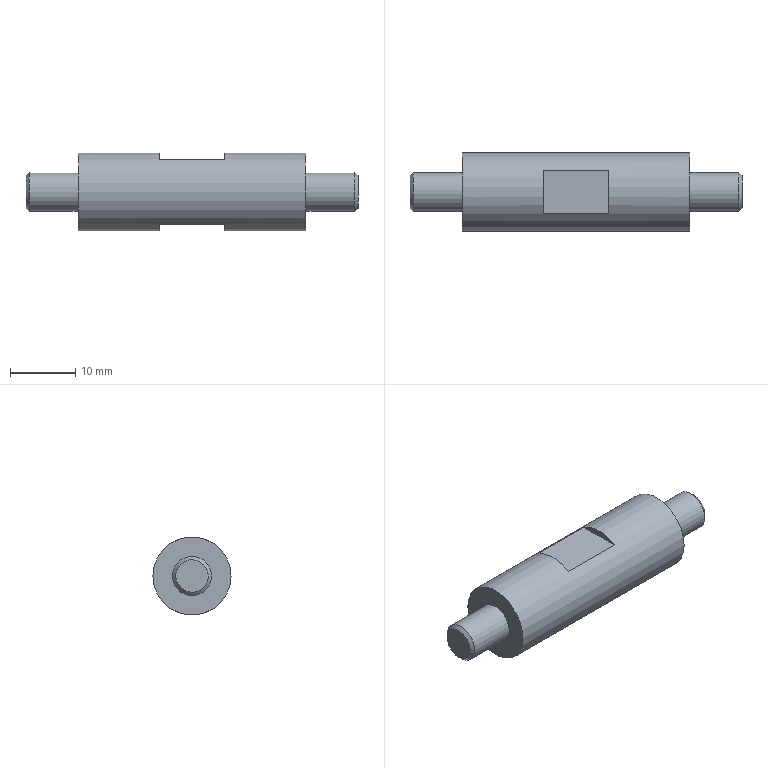Part | NX | features BREP 1 | 1 solid | 15 faces | box 51 x 12 x 12 mm | volume 4316 mm3 | plane 10 | cylinder 3 | cone 2 | commonest cylinder face diameters 6 x2 12 x1
STEP:
#1=CARTESIAN_POINT('',(17.5,-6.,0.));
#2=VERTEX_POINT('',#1);
#3=CARTESIAN_POINT('',(17.5,0.,0.));
#4=DIRECTION('',(-1.,0.,0.));
#5=DIRECTION('',(0.,-1.,0.));
#6=AXIS2_PLACEMENT_3D('',#3,#4,#5);
#7=CIRCLE('',#6,6.);
#8=EDGE_CURVE('',#2,#2,#7,.T.);
#9=ORIENTED_EDGE('',*,*,#8,.T.);
#10=EDGE_LOOP('',(#9));
#11=FACE_BOUND('',#10,.T.);
#12=CARTESIAN_POINT('',(-5.,-3.317,-5.));
#13=VERTEX_POINT('',#12);
#14=CARTESIAN_POINT('',(5.,-3.317,-5.));
#15=VERTEX_POINT('',#14);
#16=CARTESIAN_POINT('',(-25.5,-3.317,-5.));
#17=DIRECTION('',(1.,0.,0.));
#18=VECTOR('',#17,1000.);
#19=LINE('',#16,#18);
#20=EDGE_CURVE('',#13,#15,#19,.T.);
#21=ORIENTED_EDGE('',*,*,#20,.T.);
#22=CARTESIAN_POINT('',(5.,3.317,-5.));
#23=VERTEX_POINT('',#22);
#24=CARTESIAN_POINT('',(5.,0.,0.));
#25=DIRECTION('',(1.,0.,0.));
#26=DIRECTION('',(0.,-1.,0.));
#27=AXIS2_PLACEMENT_3D('',#24,#25,#26);
#28=CIRCLE('',#27,6.);
#29=EDGE_CURVE('',#15,#23,#28,.T.);
#30=ORIENTED_EDGE('',*,*,#29,.T.);
#31=CARTESIAN_POINT('',(-5.,3.317,-5.));
#32=VERTEX_POINT('',#31);
#33=CARTESIAN_POINT('',(-25.5,3.317,-5.));
#34=DIRECTION('',(-1.,0.,0.));
#35=VECTOR('',#34,1000.);
#36=LINE('',#33,#35);
#37=EDGE_CURVE('',#23,#32,#36,.T.);
#38=ORIENTED_EDGE('',*,*,#37,.T.);
#39=CARTESIAN_POINT('',(-5.,0.,0.));
#40=DIRECTION('',(-1.,0.,0.));
#41=DIRECTION('',(0.,-1.,0.));
#42=AXIS2_PLACEMENT_3D('',#39,#40,#41);
#43=CIRCLE('',#42,6.);
#44=EDGE_CURVE('',#32,#13,#43,.T.);
#45=ORIENTED_EDGE('',*,*,#44,.T.);
#46=EDGE_LOOP('',(#21,#30,#38,#45));
#47=FACE_BOUND('',#46,.T.);
#48=CARTESIAN_POINT('',(-17.5,-6.,0.));
#49=VERTEX_POINT('',#48);
#50=CARTESIAN_POINT('',(-17.5,0.,0.));
#51=DIRECTION('',(1.,0.,0.));
#52=DIRECTION('',(0.,-1.,0.));
#53=AXIS2_PLACEMENT_3D('',#50,#51,#52);
#54=CIRCLE('',#53,6.);
#55=EDGE_CURVE('',#49,#49,#54,.T.);
#56=ORIENTED_EDGE('',*,*,#55,.T.);
#57=EDGE_LOOP('',(#56));
#58=FACE_BOUND('',#57,.T.);
#59=CARTESIAN_POINT('',(5.,3.317,5.));
#60=VERTEX_POINT('',#59);
#61=CARTESIAN_POINT('',(5.,-3.317,5.));
#62=VERTEX_POINT('',#61);
#63=CARTESIAN_POINT('',(5.,0.,0.));
#64=DIRECTION('',(1.,0.,0.));
#65=DIRECTION('',(0.,-1.,0.));
#66=AXIS2_PLACEMENT_3D('',#63,#64,#65);
#67=CIRCLE('',#66,6.);
#68=EDGE_CURVE('',#60,#62,#67,.T.);
#69=ORIENTED_EDGE('',*,*,#68,.T.);
#70=CARTESIAN_POINT('',(-5.,-3.317,5.));
#71=VERTEX_POINT('',#70);
#72=CARTESIAN_POINT('',(-25.5,-3.317,5.));
#73=DIRECTION('',(-1.,0.,0.));
#74=VECTOR('',#73,1000.);
#75=LINE('',#72,#74);
#76=EDGE_CURVE('',#62,#71,#75,.T.);
#77=ORIENTED_EDGE('',*,*,#76,.T.);
#78=CARTESIAN_POINT('',(-5.,3.317,5.));
#79=VERTEX_POINT('',#78);
#80=CARTESIAN_POINT('',(-5.,0.,0.));
#81=DIRECTION('',(-1.,0.,0.));
#82=DIRECTION('',(0.,-1.,0.));
#83=AXIS2_PLACEMENT_3D('',#80,#81,#82);
#84=CIRCLE('',#83,6.);
#85=EDGE_CURVE('',#71,#79,#84,.T.);
#86=ORIENTED_EDGE('',*,*,#85,.T.);
#87=CARTESIAN_POINT('',(-25.5,3.317,5.));
#88=DIRECTION('',(1.,0.,0.));
#89=VECTOR('',#88,1000.);
#90=LINE('',#87,#89);
#91=EDGE_CURVE('',#79,#60,#90,.T.);
#92=ORIENTED_EDGE('',*,*,#91,.T.);
#93=EDGE_LOOP('',(#69,#77,#86,#92));
#94=FACE_BOUND('',#93,.T.);
#95=CARTESIAN_POINT('',(-25.5,0.,0.));
#96=DIRECTION('',(-1.,0.,0.));
#97=DIRECTION('',(0.,1.,0.));
#98=AXIS2_PLACEMENT_3D('',#95,#96,#97);
#99=CYLINDRICAL_SURFACE('',#98,6.);
#100=ADVANCED_FACE('',(#11,#47,#58,#94),#99,.T.);
#101=ORIENTED_EDGE('',*,*,#29,.F.);
#102=CARTESIAN_POINT('',(5.,0.,-5.));
#103=DIRECTION('',(0.,1.,0.));
#104=VECTOR('',#103,1000.);
#105=LINE('',#102,#104);
#106=EDGE_CURVE('',#15,#23,#105,.T.);
#107=ORIENTED_EDGE('',*,*,#106,.T.);
#108=EDGE_LOOP('',(#101,#107));
#109=FACE_BOUND('',#108,.T.);
#110=CARTESIAN_POINT('',(5.,0.,0.));
#111=DIRECTION('',(-1.,0.,0.));
#112=DIRECTION('',(0.,0.,-1.));
#113=AXIS2_PLACEMENT_3D('',#110,#111,#112);
#114=PLANE('',#113);
#115=ADVANCED_FACE('',(#109),#114,.T.);
#116=ORIENTED_EDGE('',*,*,#20,.F.);
#117=CARTESIAN_POINT('',(-5.,6.286,-5.));
#118=DIRECTION('',(0.,-1.,0.));
#119=VECTOR('',#118,1000.);
#120=LINE('',#117,#119);
#121=EDGE_CURVE('',#32,#13,#120,.T.);
#122=ORIENTED_EDGE('',*,*,#121,.F.);
#123=ORIENTED_EDGE('',*,*,#37,.F.);
#124=ORIENTED_EDGE('',*,*,#106,.F.);
#125=EDGE_LOOP('',(#116,#122,#123,#124));
#126=FACE_BOUND('',#125,.T.);
#127=CARTESIAN_POINT('',(-5.,6.286,-5.));
#128=DIRECTION('',(0.,0.,1.));
#129=DIRECTION('',(-1.,0.,0.));
#130=AXIS2_PLACEMENT_3D('',#127,#128,#129);
#131=PLANE('',#130);
#132=ADVANCED_FACE('',(#126),#131,.F.);
#133=ORIENTED_EDGE('',*,*,#44,.F.);
#134=ORIENTED_EDGE('',*,*,#121,.T.);
#135=EDGE_LOOP('',(#133,#134));
#136=FACE_BOUND('',#135,.T.);
#137=CARTESIAN_POINT('',(-5.,0.,0.));
#138=DIRECTION('',(-1.,0.,0.));
#139=DIRECTION('',(0.,0.,-1.));
#140=AXIS2_PLACEMENT_3D('',#137,#138,#139);
#141=PLANE('',#140);
#142=ADVANCED_FACE('',(#136),#141,.F.);
#143=ORIENTED_EDGE('',*,*,#55,.F.);
#144=EDGE_LOOP('',(#143));
#145=FACE_BOUND('',#144,.T.);
#146=CARTESIAN_POINT('',(-17.5,-3.,0.));
#147=VERTEX_POINT('',#146);
#148=CARTESIAN_POINT('',(-17.5,0.,0.));
#149=DIRECTION('',(-1.,0.,0.));
#150=DIRECTION('',(0.,-1.,0.));
#151=AXIS2_PLACEMENT_3D('',#148,#149,#150);
#152=CIRCLE('',#151,3.);
#153=EDGE_CURVE('',#147,#147,#152,.T.);
#154=ORIENTED_EDGE('',*,*,#153,.F.);
#155=EDGE_LOOP('',(#154));
#156=FACE_BOUND('',#155,.T.);
#157=CARTESIAN_POINT('',(-17.5,6.,0.));
#158=DIRECTION('',(1.,0.,0.));
#159=DIRECTION('',(0.,-1.,0.));
#160=AXIS2_PLACEMENT_3D('',#157,#158,#159);
#161=PLANE('',#160);
#162=ADVANCED_FACE('',(#145,#156),#161,.F.);
#163=CARTESIAN_POINT('',(17.5,-3.,0.));
#164=VERTEX_POINT('',#163);
#165=CARTESIAN_POINT('',(17.5,0.,0.));
#166=DIRECTION('',(1.,0.,0.));
#167=DIRECTION('',(0.,-1.,0.));
#168=AXIS2_PLACEMENT_3D('',#165,#166,#167);
#169=CIRCLE('',#168,3.);
#170=EDGE_CURVE('',#164,#164,#169,.T.);
#171=ORIENTED_EDGE('',*,*,#170,.F.);
#172=EDGE_LOOP('',(#171));
#173=FACE_BOUND('',#172,.T.);
#174=ORIENTED_EDGE('',*,*,#8,.F.);
#175=EDGE_LOOP('',(#174));
#176=FACE_BOUND('',#175,.T.);
#177=CARTESIAN_POINT('',(17.5,3.,0.));
#178=DIRECTION('',(-1.,0.,0.));
#179=DIRECTION('',(0.,1.,0.));
#180=AXIS2_PLACEMENT_3D('',#177,#178,#179);
#181=PLANE('',#180);
#182=ADVANCED_FACE('',(#173,#176),#181,.F.);
#183=CARTESIAN_POINT('',(-25.,-3.,0.));
#184=VERTEX_POINT('',#183);
#185=CARTESIAN_POINT('',(-25.,0.,0.));
#186=DIRECTION('',(1.,0.,0.));
#187=DIRECTION('',(0.,-1.,0.));
#188=AXIS2_PLACEMENT_3D('',#185,#186,#187);
#189=CIRCLE('',#188,3.);
#190=EDGE_CURVE('',#184,#184,#189,.T.);
#191=ORIENTED_EDGE('',*,*,#190,.T.);
#192=EDGE_LOOP('',(#191));
#193=FACE_BOUND('',#192,.T.);
#194=ORIENTED_EDGE('',*,*,#153,.T.);
#195=EDGE_LOOP('',(#194));
#196=FACE_BOUND('',#195,.T.);
#197=CARTESIAN_POINT('',(-25.5,0.,0.));
#198=DIRECTION('',(-1.,0.,0.));
#199=DIRECTION('',(0.,1.,0.));
#200=AXIS2_PLACEMENT_3D('',#197,#198,#199);
#201=CYLINDRICAL_SURFACE('',#200,3.);
#202=ADVANCED_FACE('',(#193,#196),#201,.T.);
#203=ORIENTED_EDGE('',*,*,#91,.F.);
#204=CARTESIAN_POINT('',(-5.,6.286,5.));
#205=DIRECTION('',(0.,1.,0.));
#206=VECTOR('',#205,1000.);
#207=LINE('',#204,#206);
#208=EDGE_CURVE('',#71,#79,#207,.T.);
#209=ORIENTED_EDGE('',*,*,#208,.F.);
#210=ORIENTED_EDGE('',*,*,#76,.F.);
#211=CARTESIAN_POINT('',(5.,6.286,5.));
#212=DIRECTION('',(0.,-1.,0.));
#213=VECTOR('',#212,1000.);
#214=LINE('',#211,#213);
#215=EDGE_CURVE('',#60,#62,#214,.T.);
#216=ORIENTED_EDGE('',*,*,#215,.F.);
#217=EDGE_LOOP('',(#203,#209,#210,#216));
#218=FACE_BOUND('',#217,.T.);
#219=CARTESIAN_POINT('',(-5.,6.286,5.));
#220=DIRECTION('',(0.,0.,-1.));
#221=DIRECTION('',(1.,0.,0.));
#222=AXIS2_PLACEMENT_3D('',#219,#220,#221);
#223=PLANE('',#222);
#224=ADVANCED_FACE('',(#218),#223,.F.);
#225=ORIENTED_EDGE('',*,*,#68,.F.);
#226=ORIENTED_EDGE('',*,*,#215,.T.);
#227=EDGE_LOOP('',(#225,#226));
#228=FACE_BOUND('',#227,.T.);
#229=CARTESIAN_POINT('',(5.,0.,0.));
#230=DIRECTION('',(1.,0.,0.));
#231=DIRECTION('',(0.,0.,1.));
#232=AXIS2_PLACEMENT_3D('',#229,#230,#231);
#233=PLANE('',#232);
#234=ADVANCED_FACE('',(#228),#233,.F.);
#235=ORIENTED_EDGE('',*,*,#85,.F.);
#236=ORIENTED_EDGE('',*,*,#208,.T.);
#237=EDGE_LOOP('',(#235,#236));
#238=FACE_BOUND('',#237,.T.);
#239=CARTESIAN_POINT('',(-5.,0.,0.));
#240=DIRECTION('',(1.,0.,0.));
#241=DIRECTION('',(0.,0.,1.));
#242=AXIS2_PLACEMENT_3D('',#239,#240,#241);
#243=PLANE('',#242);
#244=ADVANCED_FACE('',(#238),#243,.T.);
#245=ORIENTED_EDGE('',*,*,#170,.T.);
#246=EDGE_LOOP('',(#245));
#247=FACE_BOUND('',#246,.T.);
#248=CARTESIAN_POINT('',(25.,-3.,0.));
#249=VERTEX_POINT('',#248);
#250=CARTESIAN_POINT('',(25.,0.,0.));
#251=DIRECTION('',(-1.,0.,0.));
#252=DIRECTION('',(0.,-1.,0.));
#253=AXIS2_PLACEMENT_3D('',#250,#251,#252);
#254=CIRCLE('',#253,3.);
#255=EDGE_CURVE('',#249,#249,#254,.T.);
#256=ORIENTED_EDGE('',*,*,#255,.T.);
#257=EDGE_LOOP('',(#256));
#258=FACE_BOUND('',#257,.T.);
#259=CARTESIAN_POINT('',(-25.5,0.,0.));
#260=DIRECTION('',(-1.,0.,0.));
#261=DIRECTION('',(0.,1.,0.));
#262=AXIS2_PLACEMENT_3D('',#259,#260,#261);
#263=CYLINDRICAL_SURFACE('',#262,3.);
#264=ADVANCED_FACE('',(#247,#258),#263,.T.);
#265=ORIENTED_EDGE('',*,*,#190,.F.);
#266=EDGE_LOOP('',(#265));
#267=FACE_BOUND('',#266,.T.);
#268=CARTESIAN_POINT('',(-25.5,0.,-2.5));
#269=VERTEX_POINT('',#268);
#270=CARTESIAN_POINT('',(-25.5,0.,0.));
#271=DIRECTION('',(1.,0.,0.));
#272=DIRECTION('',(0.,0.,-1.));
#273=AXIS2_PLACEMENT_3D('',#270,#271,#272);
#274=CIRCLE('',#273,2.5);
#275=EDGE_CURVE('',#269,#269,#274,.T.);
#276=ORIENTED_EDGE('',*,*,#275,.T.);
#277=EDGE_LOOP('',(#276));
#278=FACE_BOUND('',#277,.T.);
#279=CARTESIAN_POINT('',(-25.,0.,0.));
#280=DIRECTION('',(1.,0.,0.));
#281=DIRECTION('',(0.,0.,1.));
#282=AXIS2_PLACEMENT_3D('',#279,#280,#281);
#283=CONICAL_SURFACE('',#282,3.,0.7854);
#284=ADVANCED_FACE('',(#267,#278),#283,.T.);
#285=ORIENTED_EDGE('',*,*,#255,.F.);
#286=EDGE_LOOP('',(#285));
#287=FACE_BOUND('',#286,.T.);
#288=CARTESIAN_POINT('',(25.5,0.,2.5));
#289=VERTEX_POINT('',#288);
#290=CARTESIAN_POINT('',(25.5,0.,0.));
#291=DIRECTION('',(-1.,0.,0.));
#292=DIRECTION('',(0.,0.,1.));
#293=AXIS2_PLACEMENT_3D('',#290,#291,#292);
#294=CIRCLE('',#293,2.5);
#295=EDGE_CURVE('',#289,#289,#294,.T.);
#296=ORIENTED_EDGE('',*,*,#295,.T.);
#297=EDGE_LOOP('',(#296));
#298=FACE_BOUND('',#297,.T.);
#299=CARTESIAN_POINT('',(25.,0.,0.));
#300=DIRECTION('',(-1.,0.,0.));
#301=DIRECTION('',(0.,0.,-1.));
#302=AXIS2_PLACEMENT_3D('',#299,#300,#301);
#303=CONICAL_SURFACE('',#302,3.,0.7854);
#304=ADVANCED_FACE('',(#287,#298),#303,.T.);
#305=ORIENTED_EDGE('',*,*,#275,.F.);
#306=EDGE_LOOP('',(#305));
#307=FACE_BOUND('',#306,.T.);
#308=CARTESIAN_POINT('',(-25.5,3.,0.));
#309=DIRECTION('',(1.,0.,0.));
#310=DIRECTION('',(0.,-1.,0.));
#311=AXIS2_PLACEMENT_3D('',#308,#309,#310);
#312=PLANE('',#311);
#313=ADVANCED_FACE('',(#307),#312,.F.);
#314=ORIENTED_EDGE('',*,*,#295,.F.);
#315=EDGE_LOOP('',(#314));
#316=FACE_BOUND('',#315,.T.);
#317=CARTESIAN_POINT('',(25.5,0.,0.));
#318=DIRECTION('',(-1.,0.,0.));
#319=DIRECTION('',(0.,1.,0.));
#320=AXIS2_PLACEMENT_3D('',#317,#318,#319);
#321=PLANE('',#320);
#322=ADVANCED_FACE('',(#316),#321,.F.);
#323=CLOSED_SHELL('',(#100,#115,#132,#142,#162,#182,#202,#224,#234,#244,#264,#284,#304,#313,#322));
#324=MANIFOLD_SOLID_BREP('',#323);
#325=(LENGTH_UNIT()NAMED_UNIT(*)SI_UNIT(.MILLI.,.METRE.));
#326=UNCERTAINTY_MEASURE_WITH_UNIT(LENGTH_MEASURE(0.00001),#325,'','');
#327=(NAMED_UNIT(*)PLANE_ANGLE_UNIT()SI_UNIT($,.RADIAN.));
#328=(NAMED_UNIT(*)SI_UNIT($,.STERADIAN.)SOLID_ANGLE_UNIT());
#329=(GEOMETRIC_REPRESENTATION_CONTEXT(3)GLOBAL_UNCERTAINTY_ASSIGNED_CONTEXT((#326))GLOBAL_UNIT_ASSIGNED_CONTEXT((#325,#327,#328))REPRESENTATION_CONTEXT('',''));
#330=ADVANCED_BREP_SHAPE_REPRESENTATION('',(#324),#329);